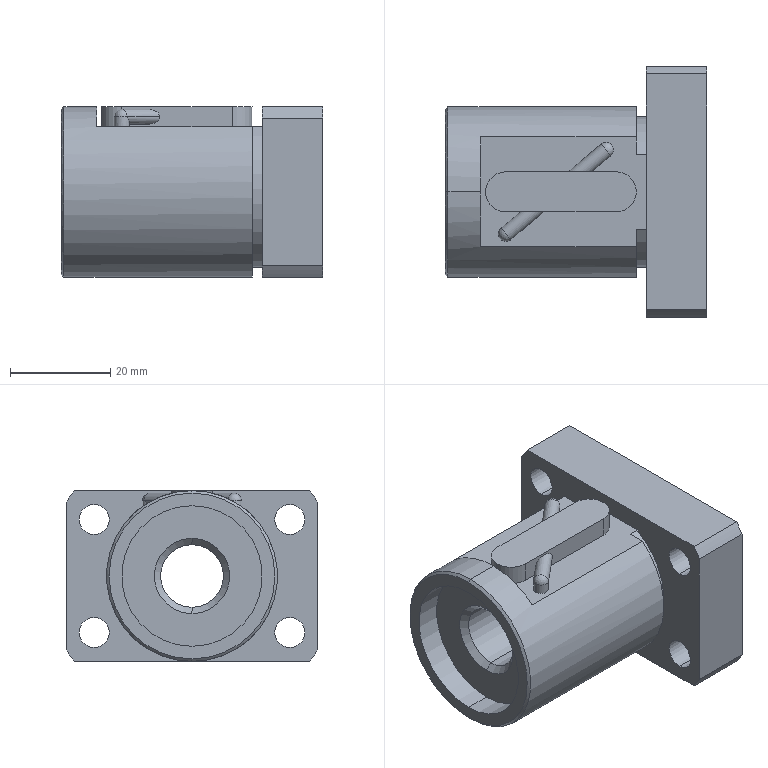Part | NX | features BREP 1 | 1 solid | 68 faces | box 52 x 50 x 34 mm | volume 41592 mm3 | cylinder 41 | plane 19 | cone 6 | sphere 2 | commonest cylinder face diameters 3 x8 6 x8 9.5 x8 28 x4 58 x4 8 x3